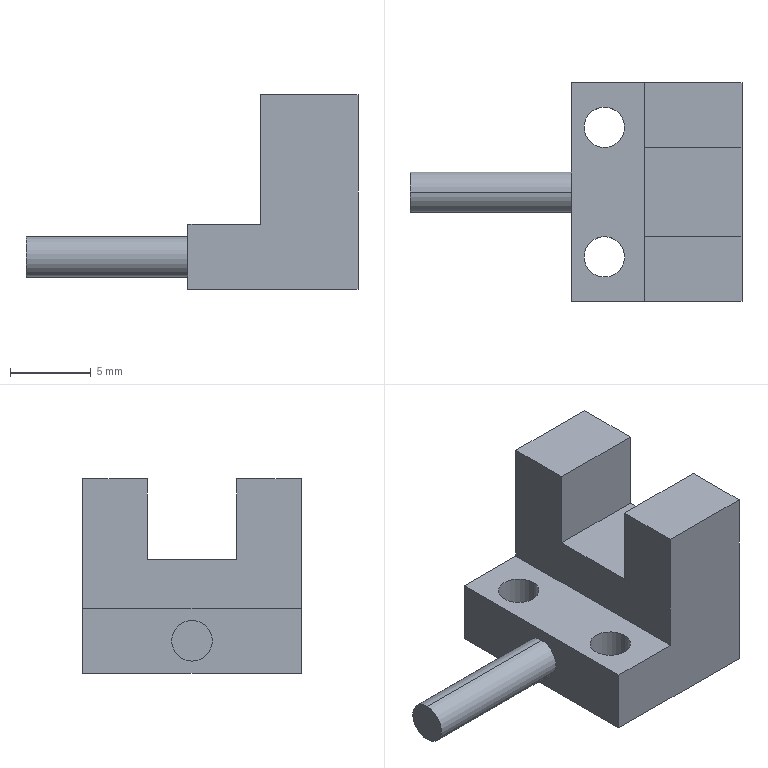Part | STEP file | 1 solid | 19 faces | box 20.5 x 13.5 x 12 mm | volume 1060 mm3 | plane 13 | cylinder 6 | commonest cylinder face diameters 2.5 x6
STEP:
#1=CARTESIAN_POINT('',(-2.,4.,-6.));
#2=VERTEX_POINT('',#1);
#3=CARTESIAN_POINT('',(-4.5,4.,-6.));
#4=VERTEX_POINT('',#3);
#5=CARTESIAN_POINT('',(-3.25,4.,-6.));
#6=DIRECTION('',(0.,0.,-1.));
#7=DIRECTION('',(1.,0.,0.));
#8=AXIS2_PLACEMENT_3D('',#5,#6,#7);
#9=CIRCLE('',#8,1.25);
#10=EDGE_CURVE('',#2,#4,#9,.T.);
#11=ORIENTED_EDGE('',*,*,#10,.T.);
#12=CARTESIAN_POINT('',(-4.5,4.,-2.));
#13=VERTEX_POINT('',#12);
#14=CARTESIAN_POINT('',(-4.5,4.,-14.));
#15=DIRECTION('',(0.,0.,1.));
#16=VECTOR('',#15,1000.);
#17=LINE('',#14,#16);
#18=EDGE_CURVE('',#4,#13,#17,.T.);
#19=ORIENTED_EDGE('',*,*,#18,.T.);
#20=CARTESIAN_POINT('',(-2.,4.,-2.));
#21=VERTEX_POINT('',#20);
#22=CARTESIAN_POINT('',(-3.25,4.,-2.));
#23=DIRECTION('',(0.,0.,1.));
#24=DIRECTION('',(1.,0.,0.));
#25=AXIS2_PLACEMENT_3D('',#22,#23,#24);
#26=CIRCLE('',#25,1.25);
#27=EDGE_CURVE('',#13,#21,#26,.T.);
#28=ORIENTED_EDGE('',*,*,#27,.T.);
#29=CARTESIAN_POINT('',(-2.,4.,-14.));
#30=DIRECTION('',(0.,0.,1.));
#31=VECTOR('',#30,1000.);
#32=LINE('',#29,#31);
#33=EDGE_CURVE('',#2,#21,#32,.T.);
#34=ORIENTED_EDGE('',*,*,#33,.F.);
#35=EDGE_LOOP('',(#11,#19,#28,#34));
#36=FACE_OUTER_BOUND('',#35,.T.);
#37=CARTESIAN_POINT('',(-3.25,4.,-14.));
#38=DIRECTION('',(0.,0.,1.));
#39=DIRECTION('',(1.,0.,0.));
#40=AXIS2_PLACEMENT_3D('',#37,#38,#39);
#41=CYLINDRICAL_SURFACE('',#40,1.25);
#42=ADVANCED_FACE('',(#36),#41,.F.);
#43=CARTESIAN_POINT('',(-2.,-4.,-6.));
#44=VERTEX_POINT('',#43);
#45=CARTESIAN_POINT('',(-4.5,-4.,-6.));
#46=VERTEX_POINT('',#45);
#47=CARTESIAN_POINT('',(-3.25,-4.,-6.));
#48=DIRECTION('',(0.,0.,-1.));
#49=DIRECTION('',(1.,0.,0.));
#50=AXIS2_PLACEMENT_3D('',#47,#48,#49);
#51=CIRCLE('',#50,1.25);
#52=EDGE_CURVE('',#44,#46,#51,.T.);
#53=ORIENTED_EDGE('',*,*,#52,.T.);
#54=CARTESIAN_POINT('',(-4.5,-4.,-2.));
#55=VERTEX_POINT('',#54);
#56=CARTESIAN_POINT('',(-4.5,-4.,-14.));
#57=DIRECTION('',(0.,0.,1.));
#58=VECTOR('',#57,1000.);
#59=LINE('',#56,#58);
#60=EDGE_CURVE('',#46,#55,#59,.T.);
#61=ORIENTED_EDGE('',*,*,#60,.T.);
#62=CARTESIAN_POINT('',(-2.,-4.,-2.));
#63=VERTEX_POINT('',#62);
#64=CARTESIAN_POINT('',(-3.25,-4.,-2.));
#65=DIRECTION('',(0.,0.,1.));
#66=DIRECTION('',(1.,0.,0.));
#67=AXIS2_PLACEMENT_3D('',#64,#65,#66);
#68=CIRCLE('',#67,1.25);
#69=EDGE_CURVE('',#55,#63,#68,.T.);
#70=ORIENTED_EDGE('',*,*,#69,.T.);
#71=CARTESIAN_POINT('',(-2.,-4.,-14.));
#72=DIRECTION('',(0.,0.,1.));
#73=VECTOR('',#72,1000.);
#74=LINE('',#71,#73);
#75=EDGE_CURVE('',#44,#63,#74,.T.);
#76=ORIENTED_EDGE('',*,*,#75,.F.);
#77=EDGE_LOOP('',(#53,#61,#70,#76));
#78=FACE_OUTER_BOUND('',#77,.T.);
#79=CARTESIAN_POINT('',(-3.25,-4.,-14.));
#80=DIRECTION('',(0.,0.,1.));
#81=DIRECTION('',(1.,0.,0.));
#82=AXIS2_PLACEMENT_3D('',#79,#80,#81);
#83=CYLINDRICAL_SURFACE('',#82,1.25);
#84=ADVANCED_FACE('',(#78),#83,.F.);
#85=CARTESIAN_POINT('',(-15.25,0.,-5.25));
#86=VERTEX_POINT('',#85);
#87=CARTESIAN_POINT('',(-15.25,0.,-2.75));
#88=VERTEX_POINT('',#87);
#89=CARTESIAN_POINT('',(-15.25,0.,-4.));
#90=DIRECTION('',(1.,0.,0.));
#91=DIRECTION('',(0.,0.,-1.));
#92=AXIS2_PLACEMENT_3D('',#89,#90,#91);
#93=CIRCLE('',#92,1.25);
#94=EDGE_CURVE('',#86,#88,#93,.T.);
#95=ORIENTED_EDGE('',*,*,#94,.T.);
#96=CARTESIAN_POINT('',(-5.25,0.,-2.75));
#97=VERTEX_POINT('',#96);
#98=CARTESIAN_POINT('',(-15.25,0.,-2.75));
#99=DIRECTION('',(1.,0.,0.));
#100=VECTOR('',#99,1000.);
#101=LINE('',#98,#100);
#102=EDGE_CURVE('',#88,#97,#101,.T.);
#103=ORIENTED_EDGE('',*,*,#102,.T.);
#104=CARTESIAN_POINT('',(-5.25,0.,-5.25));
#105=VERTEX_POINT('',#104);
#106=CARTESIAN_POINT('',(-5.25,0.,-4.));
#107=DIRECTION('',(-1.,0.,0.));
#108=DIRECTION('',(0.,0.,-1.));
#109=AXIS2_PLACEMENT_3D('',#106,#107,#108);
#110=CIRCLE('',#109,1.25);
#111=EDGE_CURVE('',#97,#105,#110,.T.);
#112=ORIENTED_EDGE('',*,*,#111,.T.);
#113=CARTESIAN_POINT('',(-15.25,0.,-5.25));
#114=DIRECTION('',(1.,0.,0.));
#115=VECTOR('',#114,1000.);
#116=LINE('',#113,#115);
#117=EDGE_CURVE('',#86,#105,#116,.T.);
#118=ORIENTED_EDGE('',*,*,#117,.F.);
#119=EDGE_LOOP('',(#95,#103,#112,#118));
#120=FACE_OUTER_BOUND('',#119,.T.);
#121=CARTESIAN_POINT('',(-15.25,0.,-4.));
#122=DIRECTION('',(1.,0.,0.));
#123=DIRECTION('',(0.,0.,-1.));
#124=AXIS2_PLACEMENT_3D('',#121,#122,#123);
#125=CYLINDRICAL_SURFACE('',#124,1.25);
#126=ADVANCED_FACE('',(#120),#125,.T.);
#127=CARTESIAN_POINT('',(5.25,-2.75,1.));
#128=VERTEX_POINT('',#127);
#129=CARTESIAN_POINT('',(5.25,2.75,1.));
#130=VERTEX_POINT('',#129);
#131=CARTESIAN_POINT('',(5.25,-6.75,1.));
#132=DIRECTION('',(0.,1.,0.));
#133=VECTOR('',#132,1000.);
#134=LINE('',#131,#133);
#135=EDGE_CURVE('',#128,#130,#134,.T.);
#136=ORIENTED_EDGE('',*,*,#135,.F.);
#137=CARTESIAN_POINT('',(5.25,-2.75,6.));
#138=VERTEX_POINT('',#137);
#139=CARTESIAN_POINT('',(5.25,-2.75,6.));
#140=DIRECTION('',(0.,0.,-1.));
#141=VECTOR('',#140,1000.);
#142=LINE('',#139,#141);
#143=EDGE_CURVE('',#138,#128,#142,.T.);
#144=ORIENTED_EDGE('',*,*,#143,.F.);
#145=CARTESIAN_POINT('',(5.25,-6.75,6.));
#146=VERTEX_POINT('',#145);
#147=CARTESIAN_POINT('',(5.25,-6.75,6.));
#148=DIRECTION('',(0.,1.,0.));
#149=VECTOR('',#148,1000.);
#150=LINE('',#147,#149);
#151=EDGE_CURVE('',#146,#138,#150,.T.);
#152=ORIENTED_EDGE('',*,*,#151,.F.);
#153=CARTESIAN_POINT('',(5.25,-6.75,-6.));
#154=VERTEX_POINT('',#153);
#155=CARTESIAN_POINT('',(5.25,-6.75,6.));
#156=DIRECTION('',(0.,0.,1.));
#157=VECTOR('',#156,1000.);
#158=LINE('',#155,#157);
#159=EDGE_CURVE('',#154,#146,#158,.T.);
#160=ORIENTED_EDGE('',*,*,#159,.F.);
#161=CARTESIAN_POINT('',(5.25,6.75,-6.));
#162=VERTEX_POINT('',#161);
#163=CARTESIAN_POINT('',(5.25,-6.75,-6.));
#164=DIRECTION('',(0.,-1.,0.));
#165=VECTOR('',#164,1000.);
#166=LINE('',#163,#165);
#167=EDGE_CURVE('',#162,#154,#166,.T.);
#168=ORIENTED_EDGE('',*,*,#167,.F.);
#169=CARTESIAN_POINT('',(5.25,6.75,6.));
#170=VERTEX_POINT('',#169);
#171=CARTESIAN_POINT('',(5.25,6.75,6.));
#172=DIRECTION('',(0.,0.,-1.));
#173=VECTOR('',#172,1000.);
#174=LINE('',#171,#173);
#175=EDGE_CURVE('',#170,#162,#174,.T.);
#176=ORIENTED_EDGE('',*,*,#175,.F.);
#177=CARTESIAN_POINT('',(5.25,2.75,6.));
#178=VERTEX_POINT('',#177);
#179=CARTESIAN_POINT('',(5.25,-6.75,6.));
#180=DIRECTION('',(0.,1.,0.));
#181=VECTOR('',#180,1000.);
#182=LINE('',#179,#181);
#183=EDGE_CURVE('',#178,#170,#182,.T.);
#184=ORIENTED_EDGE('',*,*,#183,.F.);
#185=CARTESIAN_POINT('',(5.25,2.75,6.));
#186=DIRECTION('',(0.,0.,1.));
#187=VECTOR('',#186,1000.);
#188=LINE('',#185,#187);
#189=EDGE_CURVE('',#130,#178,#188,.T.);
#190=ORIENTED_EDGE('',*,*,#189,.F.);
#191=EDGE_LOOP('',(#136,#144,#152,#160,#168,#176,#184,#190));
#192=FACE_OUTER_BOUND('',#191,.T.);
#193=CARTESIAN_POINT('',(5.25,-6.75,6.));
#194=DIRECTION('',(-1.,0.,0.));
#195=DIRECTION('',(0.,0.,1.));
#196=AXIS2_PLACEMENT_3D('',#193,#194,#195);
#197=PLANE('',#196);
#198=ADVANCED_FACE('',(#192),#197,.F.);
#199=CARTESIAN_POINT('',(-0.75,2.75,6.));
#200=VERTEX_POINT('',#199);
#201=CARTESIAN_POINT('',(-5.25,2.75,6.));
#202=DIRECTION('',(1.,0.,0.));
#203=VECTOR('',#202,1000.);
#204=LINE('',#201,#203);
#205=EDGE_CURVE('',#200,#178,#204,.T.);
#206=ORIENTED_EDGE('',*,*,#205,.F.);
#207=CARTESIAN_POINT('',(-0.75,2.75,1.));
#208=VERTEX_POINT('',#207);
#209=CARTESIAN_POINT('',(-0.75,2.75,6.));
#210=DIRECTION('',(0.,0.,1.));
#211=VECTOR('',#210,1000.);
#212=LINE('',#209,#211);
#213=EDGE_CURVE('',#208,#200,#212,.T.);
#214=ORIENTED_EDGE('',*,*,#213,.F.);
#215=CARTESIAN_POINT('',(-5.25,2.75,1.));
#216=DIRECTION('',(-1.,0.,0.));
#217=VECTOR('',#216,1000.);
#218=LINE('',#215,#217);
#219=EDGE_CURVE('',#130,#208,#218,.T.);
#220=ORIENTED_EDGE('',*,*,#219,.F.);
#221=ORIENTED_EDGE('',*,*,#189,.T.);
#222=EDGE_LOOP('',(#206,#214,#220,#221));
#223=FACE_OUTER_BOUND('',#222,.T.);
#224=CARTESIAN_POINT('',(-5.25,2.75,6.));
#225=DIRECTION('',(0.,1.,0.));
#226=DIRECTION('',(0.,0.,1.));
#227=AXIS2_PLACEMENT_3D('',#224,#225,#226);
#228=PLANE('',#227);
#229=ADVANCED_FACE('',(#223),#228,.F.);
#230=ORIENTED_EDGE('',*,*,#219,.T.);
#231=CARTESIAN_POINT('',(-0.75,-2.75,1.));
#232=VERTEX_POINT('',#231);
#233=CARTESIAN_POINT('',(-0.75,2.75,1.));
#234=DIRECTION('',(0.,1.,0.));
#235=VECTOR('',#234,1000.);
#236=LINE('',#233,#235);
#237=EDGE_CURVE('',#232,#208,#236,.T.);
#238=ORIENTED_EDGE('',*,*,#237,.F.);
#239=CARTESIAN_POINT('',(-5.25,-2.75,1.));
#240=DIRECTION('',(-1.,0.,0.));
#241=VECTOR('',#240,1000.);
#242=LINE('',#239,#241);
#243=EDGE_CURVE('',#128,#232,#242,.T.);
#244=ORIENTED_EDGE('',*,*,#243,.F.);
#245=ORIENTED_EDGE('',*,*,#135,.T.);
#246=EDGE_LOOP('',(#230,#238,#244,#245));
#247=FACE_OUTER_BOUND('',#246,.T.);
#248=CARTESIAN_POINT('',(-5.25,2.75,1.));
#249=DIRECTION('',(0.,0.,-1.));
#250=DIRECTION('',(-1.,0.,0.));
#251=AXIS2_PLACEMENT_3D('',#248,#249,#250);
#252=PLANE('',#251);
#253=ADVANCED_FACE('',(#247),#252,.F.);
#254=ORIENTED_EDGE('',*,*,#243,.T.);
#255=CARTESIAN_POINT('',(-0.75,-2.75,6.));
#256=VERTEX_POINT('',#255);
#257=CARTESIAN_POINT('',(-0.75,-2.75,6.));
#258=DIRECTION('',(0.,0.,-1.));
#259=VECTOR('',#258,1000.);
#260=LINE('',#257,#259);
#261=EDGE_CURVE('',#256,#232,#260,.T.);
#262=ORIENTED_EDGE('',*,*,#261,.F.);
#263=CARTESIAN_POINT('',(-5.25,-2.75,6.));
#264=DIRECTION('',(-1.,0.,0.));
#265=VECTOR('',#264,1000.);
#266=LINE('',#263,#265);
#267=EDGE_CURVE('',#138,#256,#266,.T.);
#268=ORIENTED_EDGE('',*,*,#267,.F.);
#269=ORIENTED_EDGE('',*,*,#143,.T.);
#270=EDGE_LOOP('',(#254,#262,#268,#269));
#271=FACE_OUTER_BOUND('',#270,.T.);
#272=CARTESIAN_POINT('',(-5.25,-2.75,6.));
#273=DIRECTION('',(0.,-1.,0.));
#274=DIRECTION('',(0.,0.,-1.));
#275=AXIS2_PLACEMENT_3D('',#272,#273,#274);
#276=PLANE('',#275);
#277=ADVANCED_FACE('',(#271),#276,.F.);
#278=ORIENTED_EDGE('',*,*,#151,.T.);
#279=ORIENTED_EDGE('',*,*,#267,.T.);
#280=CARTESIAN_POINT('',(-0.75,-6.75,6.));
#281=VERTEX_POINT('',#280);
#282=CARTESIAN_POINT('',(-0.75,6.75,6.));
#283=DIRECTION('',(0.,-1.,0.));
#284=VECTOR('',#283,1000.);
#285=LINE('',#282,#284);
#286=EDGE_CURVE('',#256,#281,#285,.T.);
#287=ORIENTED_EDGE('',*,*,#286,.T.);
#288=CARTESIAN_POINT('',(-5.25,-6.75,6.));
#289=DIRECTION('',(1.,0.,0.));
#290=VECTOR('',#289,1000.);
#291=LINE('',#288,#290);
#292=EDGE_CURVE('',#281,#146,#291,.T.);
#293=ORIENTED_EDGE('',*,*,#292,.T.);
#294=EDGE_LOOP('',(#278,#279,#287,#293));
#295=FACE_OUTER_BOUND('',#294,.T.);
#296=CARTESIAN_POINT('',(-5.25,6.75,6.));
#297=DIRECTION('',(0.,0.,1.));
#298=DIRECTION('',(1.,0.,0.));
#299=AXIS2_PLACEMENT_3D('',#296,#297,#298);
#300=PLANE('',#299);
#301=ADVANCED_FACE('',(#295),#300,.T.);
#302=CARTESIAN_POINT('',(-5.25,-6.75,-2.));
#303=VERTEX_POINT('',#302);
#304=CARTESIAN_POINT('',(-0.75,-6.75,-2.));
#305=VERTEX_POINT('',#304);
#306=CARTESIAN_POINT('',(5.25,-6.75,-2.));
#307=DIRECTION('',(1.,0.,0.));
#308=VECTOR('',#307,1000.);
#309=LINE('',#306,#308);
#310=EDGE_CURVE('',#303,#305,#309,.T.);
#311=ORIENTED_EDGE('',*,*,#310,.F.);
#312=CARTESIAN_POINT('',(-5.25,-6.75,-6.));
#313=VERTEX_POINT('',#312);
#314=CARTESIAN_POINT('',(-5.25,-6.75,6.));
#315=DIRECTION('',(0.,0.,1.));
#316=VECTOR('',#315,1000.);
#317=LINE('',#314,#316);
#318=EDGE_CURVE('',#313,#303,#317,.T.);
#319=ORIENTED_EDGE('',*,*,#318,.F.);
#320=CARTESIAN_POINT('',(5.25,-6.75,-6.));
#321=DIRECTION('',(-1.,0.,0.));
#322=VECTOR('',#321,1000.);
#323=LINE('',#320,#322);
#324=EDGE_CURVE('',#154,#313,#323,.T.);
#325=ORIENTED_EDGE('',*,*,#324,.F.);
#326=ORIENTED_EDGE('',*,*,#159,.T.);
#327=ORIENTED_EDGE('',*,*,#292,.F.);
#328=CARTESIAN_POINT('',(-0.75,-6.75,6.));
#329=DIRECTION('',(0.,0.,1.));
#330=VECTOR('',#329,1000.);
#331=LINE('',#328,#330);
#332=EDGE_CURVE('',#305,#281,#331,.T.);
#333=ORIENTED_EDGE('',*,*,#332,.F.);
#334=EDGE_LOOP('',(#311,#319,#325,#326,#327,#333));
#335=FACE_OUTER_BOUND('',#334,.T.);
#336=CARTESIAN_POINT('',(5.25,-6.75,6.));
#337=DIRECTION('',(0.,1.,0.));
#338=DIRECTION('',(0.,0.,1.));
#339=AXIS2_PLACEMENT_3D('',#336,#337,#338);
#340=PLANE('',#339);
#341=ADVANCED_FACE('',(#335),#340,.F.);
#342=ORIENTED_EDGE('',*,*,#10,.F.);
#343=CARTESIAN_POINT('',(-3.25,4.,-6.));
#344=DIRECTION('',(0.,0.,-1.));
#345=DIRECTION('',(1.,0.,0.));
#346=AXIS2_PLACEMENT_3D('',#343,#344,#345);
#347=CIRCLE('',#346,1.25);
#348=EDGE_CURVE('',#4,#2,#347,.T.);
#349=ORIENTED_EDGE('',*,*,#348,.F.);
#350=EDGE_LOOP('',(#342,#349));
#351=FACE_BOUND('',#350,.T.);
#352=ORIENTED_EDGE('',*,*,#52,.F.);
#353=CARTESIAN_POINT('',(-3.25,-4.,-6.));
#354=DIRECTION('',(0.,0.,-1.));
#355=DIRECTION('',(1.,0.,0.));
#356=AXIS2_PLACEMENT_3D('',#353,#354,#355);
#357=CIRCLE('',#356,1.25);
#358=EDGE_CURVE('',#46,#44,#357,.T.);
#359=ORIENTED_EDGE('',*,*,#358,.F.);
#360=EDGE_LOOP('',(#352,#359));
#361=FACE_BOUND('',#360,.T.);
#362=ORIENTED_EDGE('',*,*,#167,.T.);
#363=ORIENTED_EDGE('',*,*,#324,.T.);
#364=CARTESIAN_POINT('',(-5.25,6.75,-6.));
#365=VERTEX_POINT('',#364);
#366=CARTESIAN_POINT('',(-5.25,6.75,-6.));
#367=DIRECTION('',(0.,-1.,0.));
#368=VECTOR('',#367,1000.);
#369=LINE('',#366,#368);
#370=EDGE_CURVE('',#365,#313,#369,.T.);
#371=ORIENTED_EDGE('',*,*,#370,.F.);
#372=CARTESIAN_POINT('',(-5.25,6.75,-6.));
#373=DIRECTION('',(-1.,0.,0.));
#374=VECTOR('',#373,1000.);
#375=LINE('',#372,#374);
#376=EDGE_CURVE('',#162,#365,#375,.T.);
#377=ORIENTED_EDGE('',*,*,#376,.F.);
#378=EDGE_LOOP('',(#362,#363,#371,#377));
#379=FACE_OUTER_BOUND('',#378,.T.);
#380=CARTESIAN_POINT('',(-5.25,6.75,-6.));
#381=DIRECTION('',(0.,0.,1.));
#382=DIRECTION('',(1.,0.,0.));
#383=AXIS2_PLACEMENT_3D('',#380,#381,#382);
#384=PLANE('',#383);
#385=ADVANCED_FACE('',(#351,#361,#379),#384,.F.);
#386=CARTESIAN_POINT('',(-0.75,6.75,6.));
#387=VERTEX_POINT('',#386);
#388=CARTESIAN_POINT('',(5.25,6.75,6.));
#389=DIRECTION('',(-1.,0.,0.));
#390=VECTOR('',#389,1000.);
#391=LINE('',#388,#390);
#392=EDGE_CURVE('',#170,#387,#391,.T.);
#393=ORIENTED_EDGE('',*,*,#392,.F.);
#394=ORIENTED_EDGE('',*,*,#175,.T.);
#395=ORIENTED_EDGE('',*,*,#376,.T.);
#396=CARTESIAN_POINT('',(-5.25,6.75,-2.));
#397=VERTEX_POINT('',#396);
#398=CARTESIAN_POINT('',(-5.25,6.75,6.));
#399=DIRECTION('',(0.,0.,-1.));
#400=VECTOR('',#399,1000.);
#401=LINE('',#398,#400);
#402=EDGE_CURVE('',#397,#365,#401,.T.);
#403=ORIENTED_EDGE('',*,*,#402,.F.);
#404=CARTESIAN_POINT('',(-0.75,6.75,-2.));
#405=VERTEX_POINT('',#404);
#406=CARTESIAN_POINT('',(5.25,6.75,-2.));
#407=DIRECTION('',(-1.,0.,0.));
#408=VECTOR('',#407,1000.);
#409=LINE('',#406,#408);
#410=EDGE_CURVE('',#405,#397,#409,.T.);
#411=ORIENTED_EDGE('',*,*,#410,.F.);
#412=CARTESIAN_POINT('',(-0.75,6.75,6.));
#413=DIRECTION('',(0.,0.,-1.));
#414=VECTOR('',#413,1000.);
#415=LINE('',#412,#414);
#416=EDGE_CURVE('',#387,#405,#415,.T.);
#417=ORIENTED_EDGE('',*,*,#416,.F.);
#418=EDGE_LOOP('',(#393,#394,#395,#403,#411,#417));
#419=FACE_OUTER_BOUND('',#418,.T.);
#420=CARTESIAN_POINT('',(5.25,6.75,6.));
#421=DIRECTION('',(0.,-1.,0.));
#422=DIRECTION('',(0.,0.,-1.));
#423=AXIS2_PLACEMENT_3D('',#420,#421,#422);
#424=PLANE('',#423);
#425=ADVANCED_FACE('',(#419),#424,.F.);
#426=CARTESIAN_POINT('',(-0.75,6.75,6.));
#427=DIRECTION('',(0.,-1.,0.));
#428=VECTOR('',#427,1000.);
#429=LINE('',#426,#428);
#430=EDGE_CURVE('',#387,#200,#429,.T.);
#431=ORIENTED_EDGE('',*,*,#430,.T.);
#432=ORIENTED_EDGE('',*,*,#205,.T.);
#433=ORIENTED_EDGE('',*,*,#183,.T.);
#434=ORIENTED_EDGE('',*,*,#392,.T.);
#435=EDGE_LOOP('',(#431,#432,#433,#434));
#436=FACE_OUTER_BOUND('',#435,.T.);
#437=CARTESIAN_POINT('',(-5.25,6.75,6.));
#438=DIRECTION('',(0.,0.,1.));
#439=DIRECTION('',(1.,0.,0.));
#440=AXIS2_PLACEMENT_3D('',#437,#438,#439);
#441=PLANE('',#440);
#442=ADVANCED_FACE('',(#436),#441,.T.);
#443=ORIENTED_EDGE('',*,*,#430,.F.);
#444=ORIENTED_EDGE('',*,*,#416,.T.);
#445=CARTESIAN_POINT('',(-0.75,6.75,-2.));
#446=DIRECTION('',(0.,1.,0.));
#447=VECTOR('',#446,1000.);
#448=LINE('',#445,#447);
#449=EDGE_CURVE('',#305,#405,#448,.T.);
#450=ORIENTED_EDGE('',*,*,#449,.F.);
#451=ORIENTED_EDGE('',*,*,#332,.T.);
#452=ORIENTED_EDGE('',*,*,#286,.F.);
#453=ORIENTED_EDGE('',*,*,#261,.T.);
#454=ORIENTED_EDGE('',*,*,#237,.T.);
#455=ORIENTED_EDGE('',*,*,#213,.T.);
#456=EDGE_LOOP('',(#443,#444,#450,#451,#452,#453,#454,#455));
#457=FACE_OUTER_BOUND('',#456,.T.);
#458=CARTESIAN_POINT('',(-0.75,6.75,6.));
#459=DIRECTION('',(1.,0.,0.));
#460=DIRECTION('',(0.,0.,-1.));
#461=AXIS2_PLACEMENT_3D('',#458,#459,#460);
#462=PLANE('',#461);
#463=ADVANCED_FACE('',(#457),#462,.F.);
#464=CARTESIAN_POINT('',(-3.25,4.,-2.));
#465=DIRECTION('',(0.,0.,1.));
#466=DIRECTION('',(1.,0.,0.));
#467=AXIS2_PLACEMENT_3D('',#464,#465,#466);
#468=CIRCLE('',#467,1.25);
#469=EDGE_CURVE('',#21,#13,#468,.T.);
#470=ORIENTED_EDGE('',*,*,#469,.F.);
#471=ORIENTED_EDGE('',*,*,#27,.F.);
#472=EDGE_LOOP('',(#470,#471));
#473=FACE_BOUND('',#472,.T.);
#474=CARTESIAN_POINT('',(-3.25,-4.,-2.));
#475=DIRECTION('',(0.,0.,1.));
#476=DIRECTION('',(1.,0.,0.));
#477=AXIS2_PLACEMENT_3D('',#474,#475,#476);
#478=CIRCLE('',#477,1.25);
#479=EDGE_CURVE('',#63,#55,#478,.T.);
#480=ORIENTED_EDGE('',*,*,#479,.F.);
#481=ORIENTED_EDGE('',*,*,#69,.F.);
#482=EDGE_LOOP('',(#480,#481));
#483=FACE_BOUND('',#482,.T.);
#484=ORIENTED_EDGE('',*,*,#410,.T.);
#485=CARTESIAN_POINT('',(-5.25,6.75,-2.));
#486=DIRECTION('',(0.,1.,0.));
#487=VECTOR('',#486,1000.);
#488=LINE('',#485,#487);
#489=EDGE_CURVE('',#303,#397,#488,.T.);
#490=ORIENTED_EDGE('',*,*,#489,.F.);
#491=ORIENTED_EDGE('',*,*,#310,.T.);
#492=ORIENTED_EDGE('',*,*,#449,.T.);
#493=EDGE_LOOP('',(#484,#490,#491,#492));
#494=FACE_OUTER_BOUND('',#493,.T.);
#495=CARTESIAN_POINT('',(-5.25,6.75,-2.));
#496=DIRECTION('',(0.,0.,-1.));
#497=DIRECTION('',(-1.,0.,0.));
#498=AXIS2_PLACEMENT_3D('',#495,#496,#497);
#499=PLANE('',#498);
#500=ADVANCED_FACE('',(#473,#483,#494),#499,.F.);
#501=CARTESIAN_POINT('',(-5.25,0.,-4.));
#502=DIRECTION('',(-1.,0.,0.));
#503=DIRECTION('',(0.,0.,-1.));
#504=AXIS2_PLACEMENT_3D('',#501,#502,#503);
#505=CIRCLE('',#504,1.25);
#506=EDGE_CURVE('',#105,#97,#505,.T.);
#507=ORIENTED_EDGE('',*,*,#506,.F.);
#508=ORIENTED_EDGE('',*,*,#111,.F.);
#509=EDGE_LOOP('',(#507,#508));
#510=FACE_BOUND('',#509,.T.);
#511=ORIENTED_EDGE('',*,*,#402,.T.);
#512=ORIENTED_EDGE('',*,*,#370,.T.);
#513=ORIENTED_EDGE('',*,*,#318,.T.);
#514=ORIENTED_EDGE('',*,*,#489,.T.);
#515=EDGE_LOOP('',(#511,#512,#513,#514));
#516=FACE_OUTER_BOUND('',#515,.T.);
#517=CARTESIAN_POINT('',(-5.25,-6.75,6.));
#518=DIRECTION('',(1.,0.,0.));
#519=DIRECTION('',(0.,0.,-1.));
#520=AXIS2_PLACEMENT_3D('',#517,#518,#519);
#521=PLANE('',#520);
#522=ADVANCED_FACE('',(#510,#516),#521,.F.);
#523=ORIENTED_EDGE('',*,*,#18,.F.);
#524=ORIENTED_EDGE('',*,*,#348,.T.);
#525=ORIENTED_EDGE('',*,*,#33,.T.);
#526=ORIENTED_EDGE('',*,*,#469,.T.);
#527=EDGE_LOOP('',(#523,#524,#525,#526));
#528=FACE_OUTER_BOUND('',#527,.T.);
#529=CARTESIAN_POINT('',(-3.25,4.,-14.));
#530=DIRECTION('',(0.,0.,1.));
#531=DIRECTION('',(1.,0.,0.));
#532=AXIS2_PLACEMENT_3D('',#529,#530,#531);
#533=CYLINDRICAL_SURFACE('',#532,1.25);
#534=ADVANCED_FACE('',(#528),#533,.F.);
#535=ORIENTED_EDGE('',*,*,#60,.F.);
#536=ORIENTED_EDGE('',*,*,#358,.T.);
#537=ORIENTED_EDGE('',*,*,#75,.T.);
#538=ORIENTED_EDGE('',*,*,#479,.T.);
#539=EDGE_LOOP('',(#535,#536,#537,#538));
#540=FACE_OUTER_BOUND('',#539,.T.);
#541=CARTESIAN_POINT('',(-3.25,-4.,-14.));
#542=DIRECTION('',(0.,0.,1.));
#543=DIRECTION('',(1.,0.,0.));
#544=AXIS2_PLACEMENT_3D('',#541,#542,#543);
#545=CYLINDRICAL_SURFACE('',#544,1.25);
#546=ADVANCED_FACE('',(#540),#545,.F.);
#547=ORIENTED_EDGE('',*,*,#102,.F.);
#548=CARTESIAN_POINT('',(-15.25,0.,-4.));
#549=DIRECTION('',(1.,0.,0.));
#550=DIRECTION('',(0.,0.,-1.));
#551=AXIS2_PLACEMENT_3D('',#548,#549,#550);
#552=CIRCLE('',#551,1.25);
#553=EDGE_CURVE('',#88,#86,#552,.T.);
#554=ORIENTED_EDGE('',*,*,#553,.T.);
#555=ORIENTED_EDGE('',*,*,#117,.T.);
#556=ORIENTED_EDGE('',*,*,#506,.T.);
#557=EDGE_LOOP('',(#547,#554,#555,#556));
#558=FACE_OUTER_BOUND('',#557,.T.);
#559=CARTESIAN_POINT('',(-15.25,0.,-4.));
#560=DIRECTION('',(1.,0.,0.));
#561=DIRECTION('',(0.,0.,-1.));
#562=AXIS2_PLACEMENT_3D('',#559,#560,#561);
#563=CYLINDRICAL_SURFACE('',#562,1.25);
#564=ADVANCED_FACE('',(#558),#563,.T.);
#565=ORIENTED_EDGE('',*,*,#94,.F.);
#566=ORIENTED_EDGE('',*,*,#553,.F.);
#567=EDGE_LOOP('',(#565,#566));
#568=FACE_OUTER_BOUND('',#567,.T.);
#569=CARTESIAN_POINT('',(-15.25,0.,-4.));
#570=DIRECTION('',(-1.,0.,0.));
#571=DIRECTION('',(0.,0.,1.));
#572=AXIS2_PLACEMENT_3D('',#569,#570,#571);
#573=PLANE('',#572);
#574=ADVANCED_FACE('',(#568),#573,.T.);
#575=CLOSED_SHELL('',(#42,#84,#126,#198,#229,#253,#277,#301,#341,#385,#425,#442,#463,#500,#522,#534,#546,#564,#574));
#576=MANIFOLD_SOLID_BREP('',#575);
#577=CARTESIAN_POINT('',(0.,0.,0.));
#578=DIRECTION('',(0.,0.,1.));
#579=DIRECTION('',(1.,0.,0.));
#580=AXIS2_PLACEMENT_3D('',#577,#578,#579);
#581=(LENGTH_UNIT()NAMED_UNIT(*)SI_UNIT(.MILLI.,.METRE.));
#582=UNCERTAINTY_MEASURE_WITH_UNIT(LENGTH_MEASURE(0.00001),#581,'','');
#583=(NAMED_UNIT(*)PLANE_ANGLE_UNIT()SI_UNIT($,.RADIAN.));
#584=(NAMED_UNIT(*)SI_UNIT($,.STERADIAN.)SOLID_ANGLE_UNIT());
#585=(GEOMETRIC_REPRESENTATION_CONTEXT(3)GLOBAL_UNCERTAINTY_ASSIGNED_CONTEXT((#582))GLOBAL_UNIT_ASSIGNED_CONTEXT((#581,#583,#584))REPRESENTATION_CONTEXT('',''));
#586=ADVANCED_BREP_SHAPE_REPRESENTATION('',(#576,#580),#585);